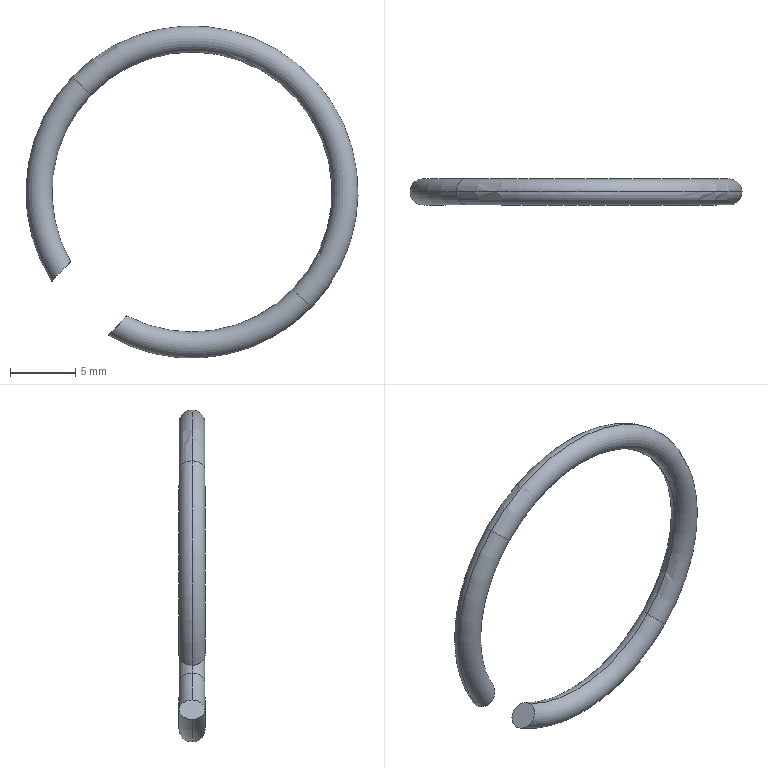Part | SolidWorks | features BaseBody 1 | 1 solid | 8 faces | box 25.5 x 2 x 25.5 mm | volume 212.875 mm3 | torus 6 | plane 2
STEP:
#1=CARTESIAN_POINT('',(220.316,126.677,8.844));
#2=VERTEX_POINT('',#1);
#3=CARTESIAN_POINT('',(221.757,126.677,7.457));
#4=VERTEX_POINT('',#3);
#5=CARTESIAN_POINT('',(221.037,126.677,8.151));
#6=DIRECTION('',(0.6937,0.,0.7203));
#7=DIRECTION('',(0.7203,0.,-0.6937));
#8=AXIS2_PLACEMENT_3D('',#5,#6,#7);
#9=CIRCLE('',#8,1.);
#10=EDGE_CURVE('',#2,#4,#9,.T.);
#11=ORIENTED_EDGE('',*,*,#10,.F.);
#12=CARTESIAN_POINT('',(218.743,126.677,-6.845));
#13=VERTEX_POINT('',#12);
#14=CARTESIAN_POINT('',(229.5,126.677,0.));
#15=DIRECTION('',(0.,-1.,0.));
#16=DIRECTION('',(0.,0.,-1.));
#17=AXIS2_PLACEMENT_3D('',#14,#15,#16);
#18=CIRCLE('',#17,12.75);
#19=EDGE_CURVE('',#2,#13,#18,.T.);
#20=ORIENTED_EDGE('',*,*,#19,.T.);
#21=CARTESIAN_POINT('',(220.178,126.677,-5.354));
#22=VERTEX_POINT('',#21);
#23=CARTESIAN_POINT('',(220.178,126.677,-5.354));
#24=CARTESIAN_POINT('',(220.178,126.545,-5.354));
#25=CARTESIAN_POINT('',(220.159,126.412,-5.374));
#26=CARTESIAN_POINT('',(220.084,126.166,-5.452));
#27=CARTESIAN_POINT('',(220.029,126.055,-5.509));
#28=CARTESIAN_POINT('',(219.896,125.873,-5.648));
#29=CARTESIAN_POINT('',(219.816,125.8,-5.731));
#30=CARTESIAN_POINT('',(219.644,125.703,-5.909));
#31=CARTESIAN_POINT('',(219.552,125.678,-6.005));
#32=CARTESIAN_POINT('',(219.274,125.677,-6.293));
#33=CARTESIAN_POINT('',(219.091,125.779,-6.483));
#34=CARTESIAN_POINT('',(218.889,126.057,-6.693));
#35=CARTESIAN_POINT('',(218.836,126.167,-6.748));
#36=CARTESIAN_POINT('',(218.762,126.411,-6.825));
#37=CARTESIAN_POINT('',(218.743,126.545,-6.845));
#38=CARTESIAN_POINT('',(218.743,126.677,-6.845));
#39=B_SPLINE_CURVE_WITH_KNOTS('',3,(#23,#24,#25,#26,#27,#28,#29,#30,#31,#32,#33,#34,#35,#36,#37,#38),.UNSPECIFIED.,.F.,.F.,(4,2,2,2,2,2,2,4),(0.00576,0.006158,0.006555,0.006952,0.007349,0.008144,0.008541,0.008939),.UNSPECIFIED.);
#40=EDGE_CURVE('',#22,#13,#39,.T.);
#41=ORIENTED_EDGE('',*,*,#40,.F.);
#42=CARTESIAN_POINT('',(229.5,126.677,0.));
#43=DIRECTION('',(0.,-1.,0.));
#44=DIRECTION('',(0.,0.,-1.));
#45=AXIS2_PLACEMENT_3D('',#42,#43,#44);
#46=CIRCLE('',#45,10.75);
#47=EDGE_CURVE('',#4,#22,#46,.T.);
#48=ORIENTED_EDGE('',*,*,#47,.F.);
#49=EDGE_LOOP('',(#11,#20,#41,#48));
#50=FACE_OUTER_BOUND('',#49,.T.);
#51=CARTESIAN_POINT('',(229.5,126.677,0.));
#52=DIRECTION('',(0.,-1.,0.));
#53=DIRECTION('',(-0.7203,0.,0.6937));
#54=AXIS2_PLACEMENT_3D('',#51,#52,#53);
#55=TOROIDAL_SURFACE('',#54,11.75,1.);
#56=ADVANCED_FACE('',(#50),#55,.T.);
#57=CARTESIAN_POINT('',(238.684,126.677,-8.844));
#58=VERTEX_POINT('',#57);
#59=CARTESIAN_POINT('',(237.243,126.677,-7.457));
#60=VERTEX_POINT('',#59);
#61=CARTESIAN_POINT('',(237.963,126.677,-8.151));
#62=DIRECTION('',(-0.6937,0.,-0.7203));
#63=DIRECTION('',(-0.7203,0.,0.6937));
#64=AXIS2_PLACEMENT_3D('',#61,#62,#63);
#65=CIRCLE('',#64,1.);
#66=EDGE_CURVE('',#58,#60,#65,.T.);
#67=ORIENTED_EDGE('',*,*,#66,.F.);
#68=CARTESIAN_POINT('',(229.5,126.677,0.));
#69=DIRECTION('',(0.,-1.,0.));
#70=DIRECTION('',(0.,0.,-1.));
#71=AXIS2_PLACEMENT_3D('',#68,#69,#70);
#72=CIRCLE('',#71,12.75);
#73=EDGE_CURVE('',#58,#2,#72,.T.);
#74=ORIENTED_EDGE('',*,*,#73,.T.);
#75=ORIENTED_EDGE('',*,*,#10,.T.);
#76=CARTESIAN_POINT('',(229.5,126.677,0.));
#77=DIRECTION('',(0.,-1.,0.));
#78=DIRECTION('',(0.,0.,-1.));
#79=AXIS2_PLACEMENT_3D('',#76,#77,#78);
#80=CIRCLE('',#79,10.75);
#81=EDGE_CURVE('',#60,#4,#80,.T.);
#82=ORIENTED_EDGE('',*,*,#81,.F.);
#83=EDGE_LOOP('',(#67,#74,#75,#82));
#84=FACE_OUTER_BOUND('',#83,.T.);
#85=CARTESIAN_POINT('',(229.5,126.677,0.));
#86=DIRECTION('',(0.,-1.,0.));
#87=DIRECTION('',(-0.7203,0.,0.6937));
#88=AXIS2_PLACEMENT_3D('',#85,#86,#87);
#89=TOROIDAL_SURFACE('',#88,11.75,1.);
#90=ADVANCED_FACE('',(#84),#89,.T.);
#91=CARTESIAN_POINT('',(223.065,126.677,-11.007));
#92=VERTEX_POINT('',#91);
#93=CARTESIAN_POINT('',(224.5,126.677,-9.516));
#94=VERTEX_POINT('',#93);
#95=CARTESIAN_POINT('',(223.065,126.677,-11.007));
#96=CARTESIAN_POINT('',(223.065,126.544,-11.007));
#97=CARTESIAN_POINT('',(223.084,126.411,-10.987));
#98=CARTESIAN_POINT('',(223.157,126.167,-10.911));
#99=CARTESIAN_POINT('',(223.212,126.055,-10.854));
#100=CARTESIAN_POINT('',(223.345,125.872,-10.716));
#101=CARTESIAN_POINT('',(223.425,125.799,-10.633));
#102=CARTESIAN_POINT('',(223.596,125.702,-10.455));
#103=CARTESIAN_POINT('',(223.689,125.677,-10.359));
#104=CARTESIAN_POINT('',(223.967,125.678,-10.07));
#105=CARTESIAN_POINT('',(224.15,125.78,-9.88));
#106=CARTESIAN_POINT('',(224.352,126.057,-9.67));
#107=CARTESIAN_POINT('',(224.406,126.168,-9.614));
#108=CARTESIAN_POINT('',(224.48,126.411,-9.537));
#109=CARTESIAN_POINT('',(224.5,126.544,-9.516));
#110=CARTESIAN_POINT('',(224.5,126.677,-9.516));
#111=B_SPLINE_CURVE_WITH_KNOTS('',3,(#95,#96,#97,#98,#99,#100,#101,#102,#103,#104,#105,#106,#107,#108,#109,#110),.UNSPECIFIED.,.F.,.F.,(4,2,2,2,2,2,2,4),(0.003783,0.004181,0.004578,0.004976,0.005373,0.006169,0.006566,0.006964),.UNSPECIFIED.);
#112=EDGE_CURVE('',#92,#94,#111,.T.);
#113=ORIENTED_EDGE('',*,*,#112,.F.);
#114=CARTESIAN_POINT('',(229.5,126.677,0.));
#115=DIRECTION('',(0.,-1.,0.));
#116=DIRECTION('',(0.,0.,-1.));
#117=AXIS2_PLACEMENT_3D('',#114,#115,#116);
#118=CIRCLE('',#117,12.75);
#119=EDGE_CURVE('',#92,#58,#118,.T.);
#120=ORIENTED_EDGE('',*,*,#119,.T.);
#121=ORIENTED_EDGE('',*,*,#66,.T.);
#122=CARTESIAN_POINT('',(229.5,126.677,0.));
#123=DIRECTION('',(0.,-1.,0.));
#124=DIRECTION('',(0.,0.,-1.));
#125=AXIS2_PLACEMENT_3D('',#122,#123,#124);
#126=CIRCLE('',#125,10.75);
#127=EDGE_CURVE('',#94,#60,#126,.T.);
#128=ORIENTED_EDGE('',*,*,#127,.F.);
#129=EDGE_LOOP('',(#113,#120,#121,#128));
#130=FACE_OUTER_BOUND('',#129,.T.);
#131=CARTESIAN_POINT('',(229.5,126.677,0.));
#132=DIRECTION('',(0.,-1.,0.));
#133=DIRECTION('',(-0.7203,0.,0.6937));
#134=AXIS2_PLACEMENT_3D('',#131,#132,#133);
#135=TOROIDAL_SURFACE('',#134,11.75,1.);
#136=ADVANCED_FACE('',(#130),#135,.T.);
#137=ORIENTED_EDGE('',*,*,#119,.F.);
#138=CARTESIAN_POINT('',(224.5,126.677,-9.516));
#139=CARTESIAN_POINT('',(224.5,126.811,-9.516));
#140=CARTESIAN_POINT('',(224.481,126.943,-9.537));
#141=CARTESIAN_POINT('',(224.406,127.189,-9.614));
#142=CARTESIAN_POINT('',(224.351,127.299,-9.671));
#143=CARTESIAN_POINT('',(224.15,127.573,-9.88));
#144=CARTESIAN_POINT('',(223.965,127.677,-10.072));
#145=CARTESIAN_POINT('',(223.689,127.678,-10.358));
#146=CARTESIAN_POINT('',(223.597,127.653,-10.455));
#147=CARTESIAN_POINT('',(223.425,127.556,-10.632));
#148=CARTESIAN_POINT('',(223.346,127.483,-10.715));
#149=CARTESIAN_POINT('',(223.212,127.299,-10.854));
#150=CARTESIAN_POINT('',(223.158,127.189,-10.91));
#151=CARTESIAN_POINT('',(223.084,126.943,-10.987));
#152=CARTESIAN_POINT('',(223.065,126.811,-11.007));
#153=CARTESIAN_POINT('',(223.065,126.677,-11.007));
#154=B_SPLINE_CURVE_WITH_KNOTS('',3,(#138,#139,#140,#141,#142,#143,#144,#145,#146,#147,#148,#149,#150,#151,#152,#153),.UNSPECIFIED.,.F.,.F.,(4,2,2,2,2,2,2,4),(0.0006011,0.0009988,0.001397,0.002192,0.00259,0.002987,0.003385,0.003783),.UNSPECIFIED.);
#155=EDGE_CURVE('',#94,#92,#154,.T.);
#156=ORIENTED_EDGE('',*,*,#155,.F.);
#157=ORIENTED_EDGE('',*,*,#127,.T.);
#158=CARTESIAN_POINT('',(237.963,126.677,-8.151));
#159=DIRECTION('',(-0.6937,0.,-0.7203));
#160=DIRECTION('',(-0.7203,0.,0.6937));
#161=AXIS2_PLACEMENT_3D('',#158,#159,#160);
#162=CIRCLE('',#161,1.);
#163=EDGE_CURVE('',#60,#58,#162,.T.);
#164=ORIENTED_EDGE('',*,*,#163,.T.);
#165=EDGE_LOOP('',(#137,#156,#157,#164));
#166=FACE_OUTER_BOUND('',#165,.T.);
#167=CARTESIAN_POINT('',(229.5,126.677,0.));
#168=DIRECTION('',(0.,-1.,0.));
#169=DIRECTION('',(-0.7203,0.,0.6937));
#170=AXIS2_PLACEMENT_3D('',#167,#168,#169);
#171=TOROIDAL_SURFACE('',#170,11.75,1.);
#172=ADVANCED_FACE('',(#166),#171,.T.);
#173=ORIENTED_EDGE('',*,*,#73,.F.);
#174=ORIENTED_EDGE('',*,*,#163,.F.);
#175=ORIENTED_EDGE('',*,*,#81,.T.);
#176=CARTESIAN_POINT('',(221.037,126.677,8.151));
#177=DIRECTION('',(0.6937,0.,0.7203));
#178=DIRECTION('',(0.7203,0.,-0.6937));
#179=AXIS2_PLACEMENT_3D('',#176,#177,#178);
#180=CIRCLE('',#179,1.);
#181=EDGE_CURVE('',#4,#2,#180,.T.);
#182=ORIENTED_EDGE('',*,*,#181,.T.);
#183=EDGE_LOOP('',(#173,#174,#175,#182));
#184=FACE_OUTER_BOUND('',#183,.T.);
#185=CARTESIAN_POINT('',(229.5,126.677,0.));
#186=DIRECTION('',(0.,-1.,0.));
#187=DIRECTION('',(-0.7203,0.,0.6937));
#188=AXIS2_PLACEMENT_3D('',#185,#186,#187);
#189=TOROIDAL_SURFACE('',#188,11.75,1.);
#190=ADVANCED_FACE('',(#184),#189,.T.);
#191=ORIENTED_EDGE('',*,*,#19,.F.);
#192=ORIENTED_EDGE('',*,*,#181,.F.);
#193=ORIENTED_EDGE('',*,*,#47,.T.);
#194=CARTESIAN_POINT('',(218.743,126.677,-6.845));
#195=CARTESIAN_POINT('',(218.743,126.81,-6.845));
#196=CARTESIAN_POINT('',(218.762,126.944,-6.825));
#197=CARTESIAN_POINT('',(218.836,127.187,-6.748));
#198=CARTESIAN_POINT('',(218.89,127.299,-6.692));
#199=CARTESIAN_POINT('',(219.091,127.575,-6.483));
#200=CARTESIAN_POINT('',(219.276,127.678,-6.292));
#201=CARTESIAN_POINT('',(219.553,127.677,-6.003));
#202=CARTESIAN_POINT('',(219.645,127.651,-5.908));
#203=CARTESIAN_POINT('',(219.817,127.554,-5.73));
#204=CARTESIAN_POINT('',(219.897,127.481,-5.647));
#205=CARTESIAN_POINT('',(220.03,127.298,-5.508));
#206=CARTESIAN_POINT('',(220.085,127.187,-5.451));
#207=CARTESIAN_POINT('',(220.159,126.944,-5.375));
#208=CARTESIAN_POINT('',(220.178,126.81,-5.354));
#209=CARTESIAN_POINT('',(220.178,126.677,-5.354));
#210=B_SPLINE_CURVE_WITH_KNOTS('',3,(#194,#195,#196,#197,#198,#199,#200,#201,#202,#203,#204,#205,#206,#207,#208,#209),.UNSPECIFIED.,.F.,.F.,(4,2,2,2,2,2,2,4),(0.00258,0.002977,0.003375,0.00417,0.004568,0.004965,0.005363,0.00576),.UNSPECIFIED.);
#211=EDGE_CURVE('',#13,#22,#210,.T.);
#212=ORIENTED_EDGE('',*,*,#211,.F.);
#213=EDGE_LOOP('',(#191,#192,#193,#212));
#214=FACE_OUTER_BOUND('',#213,.T.);
#215=CARTESIAN_POINT('',(229.5,126.677,0.));
#216=DIRECTION('',(0.,-1.,0.));
#217=DIRECTION('',(-0.7203,0.,0.6937));
#218=AXIS2_PLACEMENT_3D('',#215,#216,#217);
#219=TOROIDAL_SURFACE('',#218,11.75,1.);
#220=ADVANCED_FACE('',(#214),#219,.T.);
#221=ORIENTED_EDGE('',*,*,#155,.T.);
#222=ORIENTED_EDGE('',*,*,#112,.T.);
#223=EDGE_LOOP('',(#221,#222));
#224=FACE_OUTER_BOUND('',#223,.T.);
#225=CARTESIAN_POINT('',(224.762,127.677,-9.245));
#226=DIRECTION('',(-0.7203,0.,0.6937));
#227=DIRECTION('',(0.6937,0.,0.7203));
#228=AXIS2_PLACEMENT_3D('',#225,#226,#227);
#229=PLANE('',#228);
#230=ADVANCED_FACE('',(#224),#229,.T.);
#231=ORIENTED_EDGE('',*,*,#40,.T.);
#232=ORIENTED_EDGE('',*,*,#211,.T.);
#233=EDGE_LOOP('',(#231,#232));
#234=FACE_OUTER_BOUND('',#233,.T.);
#235=CARTESIAN_POINT('',(220.44,127.677,-5.083));
#236=DIRECTION('',(0.7203,0.,-0.6937));
#237=DIRECTION('',(-0.6937,0.,-0.7203));
#238=AXIS2_PLACEMENT_3D('',#235,#236,#237);
#239=PLANE('',#238);
#240=ADVANCED_FACE('',(#234),#239,.T.);
#241=CLOSED_SHELL('',(#56,#90,#136,#172,#190,#220,#230,#240));
#242=MANIFOLD_SOLID_BREP('',#241);
#243=CARTESIAN_POINT('',(0.,0.,0.));
#244=DIRECTION('',(0.,0.,1.));
#245=DIRECTION('',(1.,0.,0.));
#246=AXIS2_PLACEMENT_3D('',#243,#244,#245);
#247=(LENGTH_UNIT()NAMED_UNIT(*)SI_UNIT(.MILLI.,.METRE.));
#248=UNCERTAINTY_MEASURE_WITH_UNIT(LENGTH_MEASURE(0.00001),#247,'','');
#249=(NAMED_UNIT(*)PLANE_ANGLE_UNIT()SI_UNIT($,.RADIAN.));
#250=(NAMED_UNIT(*)SI_UNIT($,.STERADIAN.)SOLID_ANGLE_UNIT());
#251=(GEOMETRIC_REPRESENTATION_CONTEXT(3)GLOBAL_UNCERTAINTY_ASSIGNED_CONTEXT((#248))GLOBAL_UNIT_ASSIGNED_CONTEXT((#247,#249,#250))REPRESENTATION_CONTEXT('',''));
#252=ADVANCED_BREP_SHAPE_REPRESENTATION('',(#242,#246),#251);